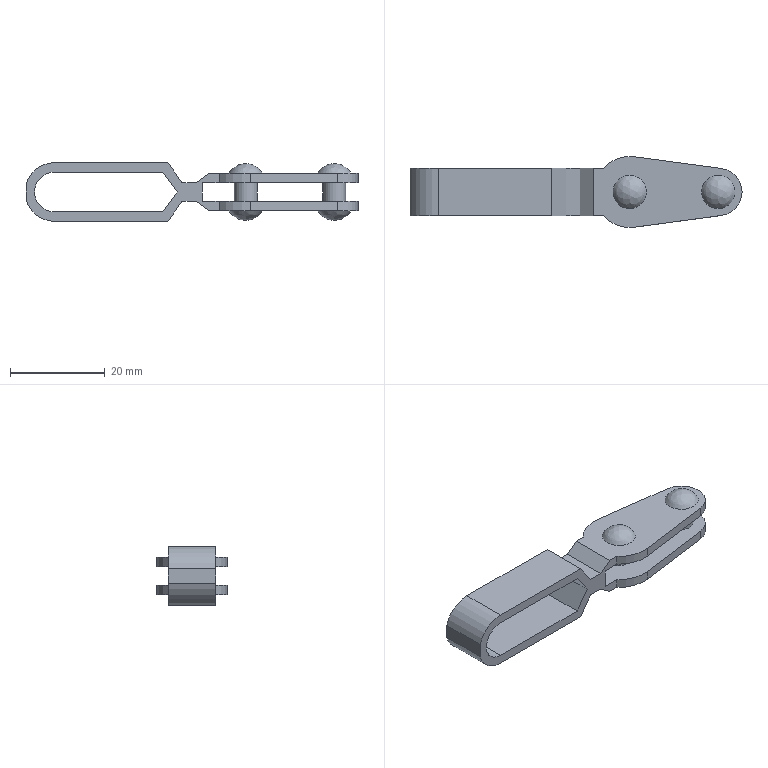Part | SolidWorks | features BaseBody 1 | 1 solid | 43 faces | box 70.05 x 15.001 x 12.4 mm | volume 3515 mm3 | plane 24 | cylinder 15 | spline 4 | commonest cylinder face diameters 4.8 x4 10 x4 15 x4 12.4 x2 8.4 x1